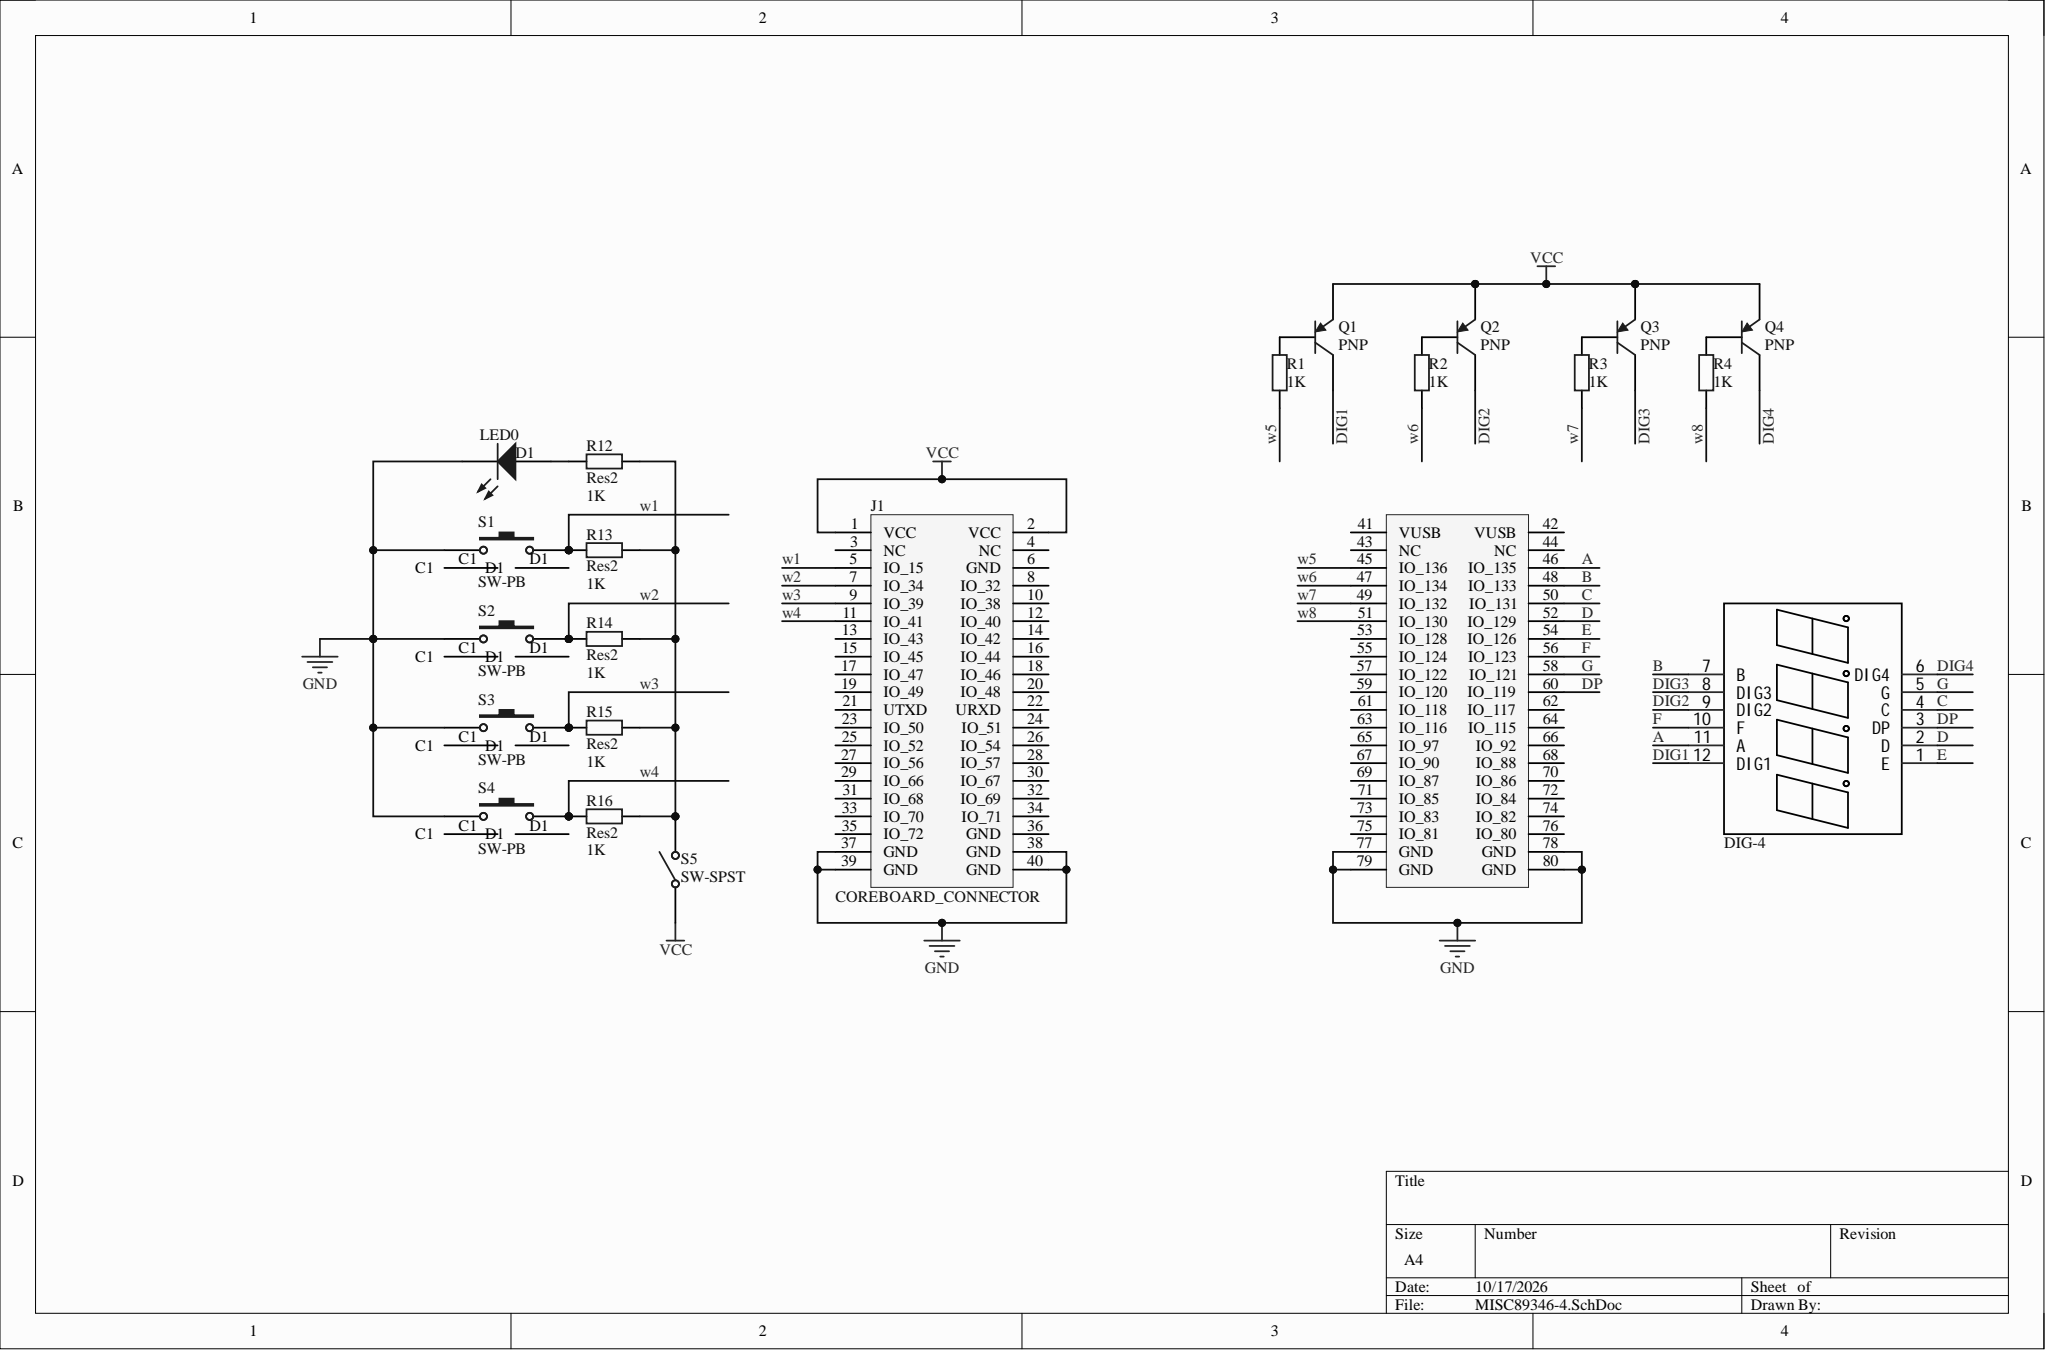Circuit board | Altium Designer | 21 parts | 24 nets
Bill of materials:
Comment,Description,Designator,Footprint,LibRef,Quantity
"DIG-4","","","DIG-4","DIG-4","1"
"LED0","Typical INFRARED GaAs LED","D1","LED_TH_HLMP4700","LED0","1"
"COREBOARD_CONNECTOR","","J1","coreboard_connector","COREBOARD_CONNECTOR","1"
"PNP","PNP Bipolar Transistor","Q1, Q2, Q3, Q4","TO-92","PNP","4"
"","Resistor","R1, R2, R3, R4","AXIAL-0.5","Res2","4"
"Res2","Resistor","R12, R13, R14, R15, R16","AXIAL-0.5","Res2","5"
"SW-PB","Switch","S1, S2, S3, S4","TS665CJ","SW-PB","4"
"SW-SPST","Single-Pole, Single-Throw Switch","S5","SS12D10","SW-SPST","1"
Netlist (Protel format):
[

DIG-4
DIG-4



]
[
D1
LED_TH_HLMP4700
LED0



]
[
J1
coreboard_connector
COREBOARD_CONNECTOR



]
[
Q1
TO-92
PNP



]
[
Q2
TO-92
PNP



]
[
Q3
TO-92
PNP



]
[
Q4
TO-92
PNP



]
[
R1
AXIAL-0.5




]
[
R2
AXIAL-0.5




]
[
R3
AXIAL-0.5




]
[
R4
AXIAL-0.5




]
[
R12
AXIAL-0.5
Res2



]
[
R13
AXIAL-0.5
Res2



]
[
R14
AXIAL-0.5
Res2



]
[
R15
AXIAL-0.5
Res2



]
[
R16
AXIAL-0.5
Res2



]
[
S1
TS665CJ
SW-PB



]
[
S2
TS665CJ
SW-PB



]
[
S3
TS665CJ
SW-PB



]
[
S4
TS665CJ
SW-PB



]
[
S5
SS12D10
SW-SPST



]
(
w8
J1-51
R4-1
)
(
w7
J1-49
R3-1
)
(
w6
J1-47
R2-1
)
(
w5
J1-45
R1-1
)
(
w4
J1-11
R16-1
S4-2
)
(
w3
J1-9
R15-1
S3-2
)
(
w2
J1-7
R14-1
S2-2
)
(
w1
J1-5
R13-1
S1-2
)
(
VCC
J1-1
J1-2
Q1-3
Q2-3
Q3-3
Q4-3
S5-1
)
(
NetR12_2
R12-2
R13-2
R14-2
R15-2
R16-2
S5-2
)
(
NetQ4_2
Q4-2
R4-2
)
(
NetQ3_2
Q3-2
R3-2
)
(
NetQ2_2
Q2-2
R2-2
)
(
NetQ1_2
Q1-2
R1-2
)
(
NetD1_1
D1-1
R12-1
)
(
GND
D1-2
J1-37
J1-38
J1-39
J1-40
J1-77
J1-78
J1-79
J1-80
S1-A1
S2-A1
S3-A1
S4-A1
)
(
G
-5
J1-58
)
(
F
-10
J1-56
)
(
E
-1
J1-54
)
(
DP
-3
J1-60
)
(
D
-2
J1-52
)
(
C
-4
J1-50
)
(
B
-7
J1-48
)
(
A
-11
J1-46
)